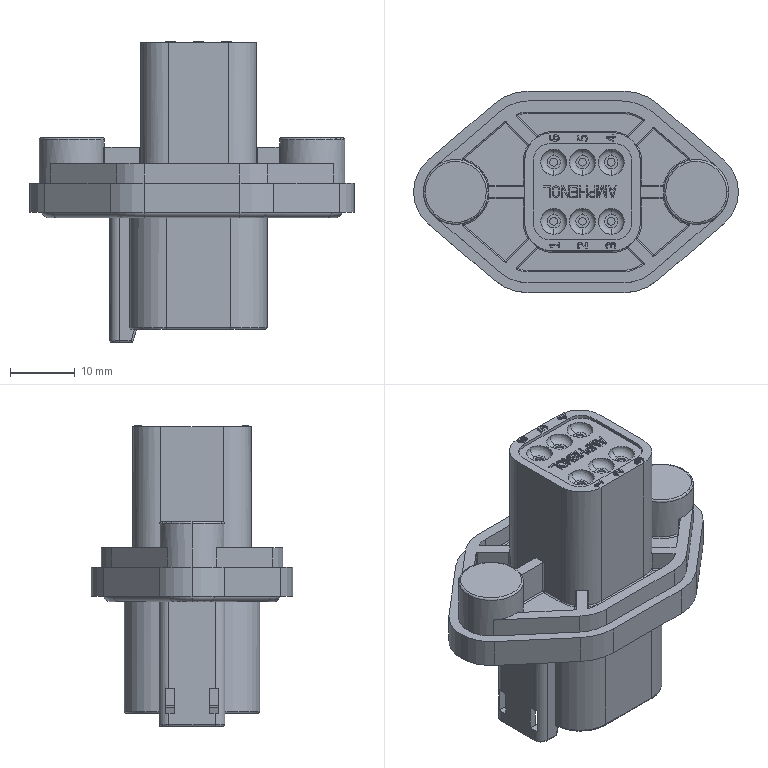Part | NX | features BREP 1 | 1 solid | 686 faces | box 50 x 31 x 46.3 mm | volume 15321 mm3 | plane 300 | cylinder 201 | spline 89 | torus 59 | sphere 23 | cone 14 | commonest cylinder face diameters 0.4 x62 3.25 x44 1.2 x12 2 x12 0.6 x9 13 x6